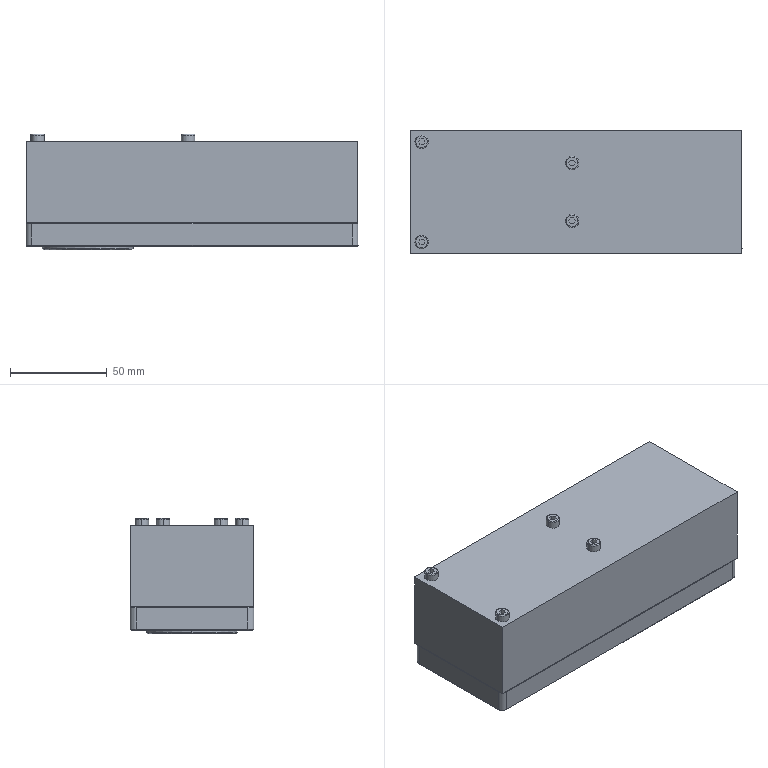Part | SolidWorks | 2 solids | 236 faces | box 172 x 64 x 60 mm | volume 126138 mm3 | plane 90 | cylinder 83 | cone 55 | spline 8 | commonest cylinder face diameters 4.5 x24 6 x16 8 x16 3.3 x12 7 x8 50 x3